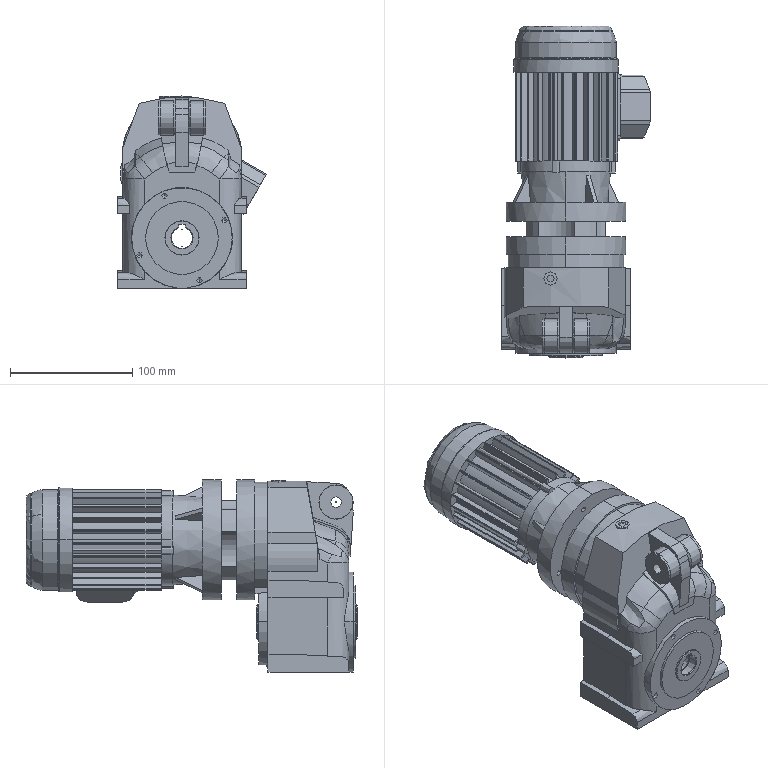Part | STEP file | 8 solids | 587 faces | box 121.404 x 271.25 x 157.01 mm | volume 2000686 mm3 | cylinder 263 | plane 261 | cone 32 | spline 31 | commonest cylinder face diameters 0.7 x47 71.4 x22 4.653 x20 82.6 x20 0.35 x18 4.2 x18